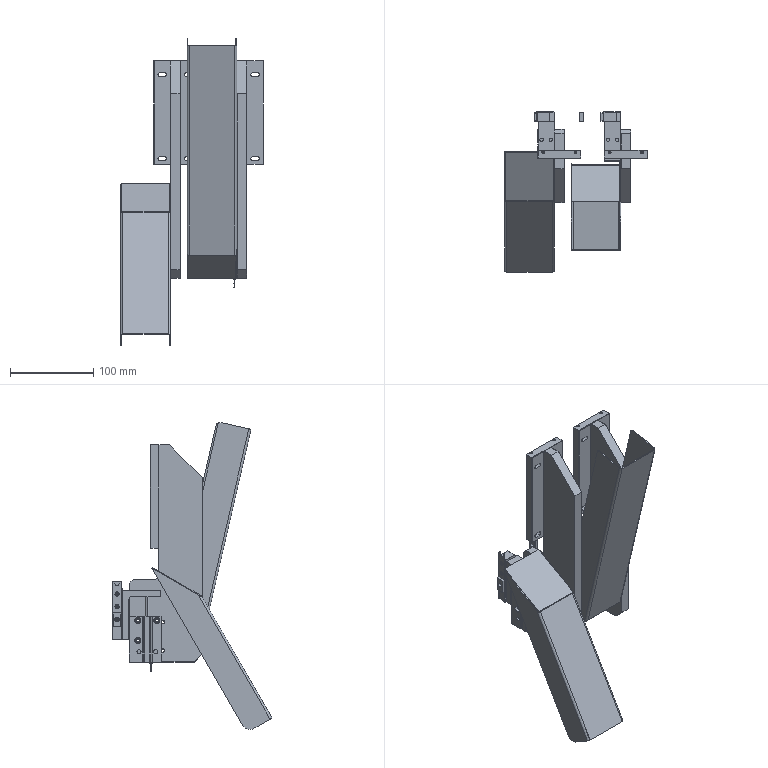Part | NX | 21 solids | 1175 faces | box 172 x 192.647 x 369.75 mm | volume 712254 mm3 | plane 500 | cylinder 499 | cone 176 | commonest cylinder face diameters 2.5 x104 4 x100 5 x84 3.3 x44 4.5 x36 7.5 x24